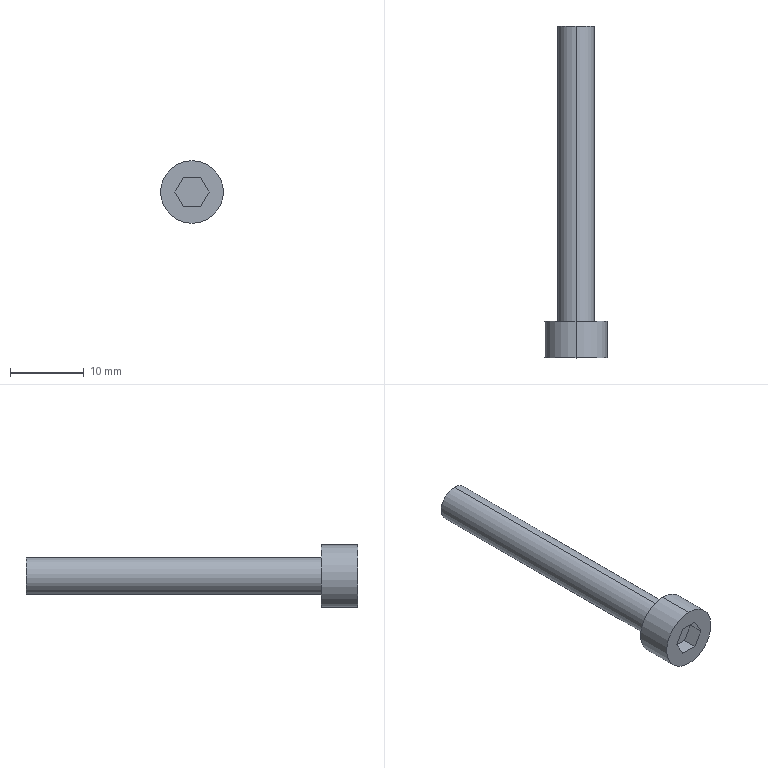Part | SolidWorks | features BaseBody 1 | 1 solid | 14 faces | box 8.5 x 45 x 8.5 mm | volume 1041 mm3 | plane 10 | cylinder 4 | commonest cylinder face diameters 5 x2 8.5 x2
STEP:
#1=CARTESIAN_POINT('',(0.,45.,-2.5));
#2=VERTEX_POINT('',#1);
#3=CARTESIAN_POINT('',(0.,45.,2.5));
#4=VERTEX_POINT('',#3);
#5=CARTESIAN_POINT('',(0.,45.,0.));
#6=DIRECTION('',(0.,-1.,0.));
#7=DIRECTION('',(0.,0.,-1.));
#8=AXIS2_PLACEMENT_3D('',#5,#6,#7);
#9=CIRCLE('',#8,2.5);
#10=EDGE_CURVE('',#2,#4,#9,.T.);
#11=ORIENTED_EDGE('',*,*,#10,.T.);
#12=CARTESIAN_POINT('',(0.,5.,2.5));
#13=VERTEX_POINT('',#12);
#14=CARTESIAN_POINT('',(0.,45.,2.5));
#15=DIRECTION('',(0.,-1.,0.));
#16=VECTOR('',#15,1000.);
#17=LINE('',#14,#16);
#18=EDGE_CURVE('',#4,#13,#17,.T.);
#19=ORIENTED_EDGE('',*,*,#18,.T.);
#20=CARTESIAN_POINT('',(0.,5.,-2.5));
#21=VERTEX_POINT('',#20);
#22=CARTESIAN_POINT('',(0.,5.,0.));
#23=DIRECTION('',(0.,1.,0.));
#24=DIRECTION('',(0.,0.,-1.));
#25=AXIS2_PLACEMENT_3D('',#22,#23,#24);
#26=CIRCLE('',#25,2.5);
#27=EDGE_CURVE('',#13,#21,#26,.T.);
#28=ORIENTED_EDGE('',*,*,#27,.T.);
#29=CARTESIAN_POINT('',(0.,45.,-2.5));
#30=DIRECTION('',(0.,-1.,0.));
#31=VECTOR('',#30,1000.);
#32=LINE('',#29,#31);
#33=EDGE_CURVE('',#2,#21,#32,.T.);
#34=ORIENTED_EDGE('',*,*,#33,.F.);
#35=EDGE_LOOP('',(#11,#19,#28,#34));
#36=FACE_OUTER_BOUND('',#35,.T.);
#37=CARTESIAN_POINT('',(0.,45.,0.));
#38=DIRECTION('',(0.,-1.,0.));
#39=DIRECTION('',(0.,0.,-1.));
#40=AXIS2_PLACEMENT_3D('',#37,#38,#39);
#41=CYLINDRICAL_SURFACE('',#40,2.5);
#42=ADVANCED_FACE('',(#36),#41,.T.);
#43=CARTESIAN_POINT('',(0.,5.,4.25));
#44=VERTEX_POINT('',#43);
#45=CARTESIAN_POINT('',(0.,5.,-4.25));
#46=VERTEX_POINT('',#45);
#47=CARTESIAN_POINT('',(0.,5.,0.));
#48=DIRECTION('',(0.,1.,0.));
#49=DIRECTION('',(0.,0.,-1.));
#50=AXIS2_PLACEMENT_3D('',#47,#48,#49);
#51=CIRCLE('',#50,4.25);
#52=EDGE_CURVE('',#44,#46,#51,.T.);
#53=ORIENTED_EDGE('',*,*,#52,.F.);
#54=CARTESIAN_POINT('',(0.,0.,4.25));
#55=VERTEX_POINT('',#54);
#56=CARTESIAN_POINT('',(0.,5.,4.25));
#57=DIRECTION('',(0.,-1.,0.));
#58=VECTOR('',#57,1000.);
#59=LINE('',#56,#58);
#60=EDGE_CURVE('',#44,#55,#59,.T.);
#61=ORIENTED_EDGE('',*,*,#60,.T.);
#62=CARTESIAN_POINT('',(0.,0.,-4.25));
#63=VERTEX_POINT('',#62);
#64=CARTESIAN_POINT('',(0.,0.,0.));
#65=DIRECTION('',(0.,1.,0.));
#66=DIRECTION('',(0.,0.,-1.));
#67=AXIS2_PLACEMENT_3D('',#64,#65,#66);
#68=CIRCLE('',#67,4.25);
#69=EDGE_CURVE('',#55,#63,#68,.T.);
#70=ORIENTED_EDGE('',*,*,#69,.T.);
#71=CARTESIAN_POINT('',(0.,5.,-4.25));
#72=DIRECTION('',(0.,-1.,0.));
#73=VECTOR('',#72,1000.);
#74=LINE('',#71,#73);
#75=EDGE_CURVE('',#46,#63,#74,.T.);
#76=ORIENTED_EDGE('',*,*,#75,.F.);
#77=EDGE_LOOP('',(#53,#61,#70,#76));
#78=FACE_OUTER_BOUND('',#77,.T.);
#79=CARTESIAN_POINT('',(0.,5.,0.));
#80=DIRECTION('',(0.,-1.,0.));
#81=DIRECTION('',(0.,0.,-1.));
#82=AXIS2_PLACEMENT_3D('',#79,#80,#81);
#83=CYLINDRICAL_SURFACE('',#82,4.25);
#84=ADVANCED_FACE('',(#78),#83,.T.);
#85=ORIENTED_EDGE('',*,*,#18,.F.);
#86=CARTESIAN_POINT('',(0.,45.,0.));
#87=DIRECTION('',(0.,-1.,0.));
#88=DIRECTION('',(0.,0.,-1.));
#89=AXIS2_PLACEMENT_3D('',#86,#87,#88);
#90=CIRCLE('',#89,2.5);
#91=EDGE_CURVE('',#4,#2,#90,.T.);
#92=ORIENTED_EDGE('',*,*,#91,.T.);
#93=ORIENTED_EDGE('',*,*,#33,.T.);
#94=CARTESIAN_POINT('',(0.,5.,0.));
#95=DIRECTION('',(0.,1.,0.));
#96=DIRECTION('',(0.,0.,-1.));
#97=AXIS2_PLACEMENT_3D('',#94,#95,#96);
#98=CIRCLE('',#97,2.5);
#99=EDGE_CURVE('',#21,#13,#98,.T.);
#100=ORIENTED_EDGE('',*,*,#99,.T.);
#101=EDGE_LOOP('',(#85,#92,#93,#100));
#102=FACE_OUTER_BOUND('',#101,.T.);
#103=CARTESIAN_POINT('',(0.,45.,0.));
#104=DIRECTION('',(0.,-1.,0.));
#105=DIRECTION('',(0.,0.,-1.));
#106=AXIS2_PLACEMENT_3D('',#103,#104,#105);
#107=CYLINDRICAL_SURFACE('',#106,2.5);
#108=ADVANCED_FACE('',(#102),#107,.T.);
#109=CARTESIAN_POINT('',(0.,5.,0.));
#110=DIRECTION('',(0.,1.,0.));
#111=DIRECTION('',(0.,0.,-1.));
#112=AXIS2_PLACEMENT_3D('',#109,#110,#111);
#113=CIRCLE('',#112,4.25);
#114=EDGE_CURVE('',#46,#44,#113,.T.);
#115=ORIENTED_EDGE('',*,*,#114,.T.);
#116=ORIENTED_EDGE('',*,*,#52,.T.);
#117=EDGE_LOOP('',(#115,#116));
#118=FACE_OUTER_BOUND('',#117,.T.);
#119=ORIENTED_EDGE('',*,*,#99,.F.);
#120=ORIENTED_EDGE('',*,*,#27,.F.);
#121=EDGE_LOOP('',(#119,#120));
#122=FACE_BOUND('',#121,.T.);
#123=CARTESIAN_POINT('',(0.,5.,0.));
#124=DIRECTION('',(0.,1.,0.));
#125=DIRECTION('',(0.,0.,1.));
#126=AXIS2_PLACEMENT_3D('',#123,#124,#125);
#127=PLANE('',#126);
#128=ADVANCED_FACE('',(#118,#122),#127,.T.);
#129=ORIENTED_EDGE('',*,*,#10,.F.);
#130=ORIENTED_EDGE('',*,*,#91,.F.);
#131=EDGE_LOOP('',(#129,#130));
#132=FACE_OUTER_BOUND('',#131,.T.);
#133=CARTESIAN_POINT('',(0.,45.,0.));
#134=DIRECTION('',(0.,1.,0.));
#135=DIRECTION('',(0.,0.,1.));
#136=AXIS2_PLACEMENT_3D('',#133,#134,#135);
#137=PLANE('',#136);
#138=ADVANCED_FACE('',(#132),#137,.T.);
#139=ORIENTED_EDGE('',*,*,#60,.F.);
#140=ORIENTED_EDGE('',*,*,#114,.F.);
#141=ORIENTED_EDGE('',*,*,#75,.T.);
#142=CARTESIAN_POINT('',(0.,0.,0.));
#143=DIRECTION('',(0.,1.,0.));
#144=DIRECTION('',(0.,0.,-1.));
#145=AXIS2_PLACEMENT_3D('',#142,#143,#144);
#146=CIRCLE('',#145,4.25);
#147=EDGE_CURVE('',#63,#55,#146,.T.);
#148=ORIENTED_EDGE('',*,*,#147,.T.);
#149=EDGE_LOOP('',(#139,#140,#141,#148));
#150=FACE_OUTER_BOUND('',#149,.T.);
#151=CARTESIAN_POINT('',(0.,5.,0.));
#152=DIRECTION('',(0.,-1.,0.));
#153=DIRECTION('',(0.,0.,-1.));
#154=AXIS2_PLACEMENT_3D('',#151,#152,#153);
#155=CYLINDRICAL_SURFACE('',#154,4.25);
#156=ADVANCED_FACE('',(#150),#155,.T.);
#157=ORIENTED_EDGE('',*,*,#147,.F.);
#158=ORIENTED_EDGE('',*,*,#69,.F.);
#159=EDGE_LOOP('',(#157,#158));
#160=FACE_OUTER_BOUND('',#159,.T.);
#161=CARTESIAN_POINT('',(1.155,0.,-2.));
#162=VERTEX_POINT('',#161);
#163=CARTESIAN_POINT('',(2.309,0.,0.));
#164=VERTEX_POINT('',#163);
#165=CARTESIAN_POINT('',(1.155,0.,-2.));
#166=DIRECTION('',(0.5,0.,0.866));
#167=VECTOR('',#166,1000.);
#168=LINE('',#165,#167);
#169=EDGE_CURVE('',#162,#164,#168,.T.);
#170=ORIENTED_EDGE('',*,*,#169,.F.);
#171=CARTESIAN_POINT('',(-1.155,0.,-2.));
#172=VERTEX_POINT('',#171);
#173=CARTESIAN_POINT('',(0.,0.,-2.));
#174=DIRECTION('',(1.,0.,0.));
#175=VECTOR('',#174,1000.);
#176=LINE('',#173,#175);
#177=EDGE_CURVE('',#172,#162,#176,.T.);
#178=ORIENTED_EDGE('',*,*,#177,.F.);
#179=CARTESIAN_POINT('',(-2.309,0.,0.));
#180=VERTEX_POINT('',#179);
#181=CARTESIAN_POINT('',(-2.309,0.,0.));
#182=DIRECTION('',(0.5,0.,-0.866));
#183=VECTOR('',#182,1000.);
#184=LINE('',#181,#183);
#185=EDGE_CURVE('',#180,#172,#184,.T.);
#186=ORIENTED_EDGE('',*,*,#185,.F.);
#187=CARTESIAN_POINT('',(-1.155,0.,2.));
#188=VERTEX_POINT('',#187);
#189=CARTESIAN_POINT('',(-1.155,0.,2.));
#190=DIRECTION('',(-0.5,0.,-0.866));
#191=VECTOR('',#190,1000.);
#192=LINE('',#189,#191);
#193=EDGE_CURVE('',#188,#180,#192,.T.);
#194=ORIENTED_EDGE('',*,*,#193,.F.);
#195=CARTESIAN_POINT('',(1.155,0.,2.));
#196=VERTEX_POINT('',#195);
#197=CARTESIAN_POINT('',(0.,0.,2.));
#198=DIRECTION('',(-1.,0.,0.));
#199=VECTOR('',#198,1000.);
#200=LINE('',#197,#199);
#201=EDGE_CURVE('',#196,#188,#200,.T.);
#202=ORIENTED_EDGE('',*,*,#201,.F.);
#203=CARTESIAN_POINT('',(2.309,0.,0.));
#204=DIRECTION('',(-0.5,0.,0.866));
#205=VECTOR('',#204,1000.);
#206=LINE('',#203,#205);
#207=EDGE_CURVE('',#164,#196,#206,.T.);
#208=ORIENTED_EDGE('',*,*,#207,.F.);
#209=EDGE_LOOP('',(#170,#178,#186,#194,#202,#208));
#210=FACE_BOUND('',#209,.T.);
#211=CARTESIAN_POINT('',(0.,0.,0.));
#212=DIRECTION('',(0.,1.,0.));
#213=DIRECTION('',(0.,0.,1.));
#214=AXIS2_PLACEMENT_3D('',#211,#212,#213);
#215=PLANE('',#214);
#216=ADVANCED_FACE('',(#160,#210),#215,.F.);
#217=CARTESIAN_POINT('',(1.155,2.,2.));
#218=VERTEX_POINT('',#217);
#219=CARTESIAN_POINT('',(1.155,2.,2.));
#220=DIRECTION('',(0.,-1.,0.));
#221=VECTOR('',#220,1000.);
#222=LINE('',#219,#221);
#223=EDGE_CURVE('',#218,#196,#222,.T.);
#224=ORIENTED_EDGE('',*,*,#223,.F.);
#225=CARTESIAN_POINT('',(2.309,2.,0.));
#226=VERTEX_POINT('',#225);
#227=CARTESIAN_POINT('',(2.309,2.,0.));
#228=DIRECTION('',(-0.5,0.,0.866));
#229=VECTOR('',#228,1000.);
#230=LINE('',#227,#229);
#231=EDGE_CURVE('',#226,#218,#230,.T.);
#232=ORIENTED_EDGE('',*,*,#231,.F.);
#233=CARTESIAN_POINT('',(2.309,2.,0.));
#234=DIRECTION('',(0.,1.,0.));
#235=VECTOR('',#234,1000.);
#236=LINE('',#233,#235);
#237=EDGE_CURVE('',#164,#226,#236,.T.);
#238=ORIENTED_EDGE('',*,*,#237,.F.);
#239=ORIENTED_EDGE('',*,*,#207,.T.);
#240=EDGE_LOOP('',(#224,#232,#238,#239));
#241=FACE_OUTER_BOUND('',#240,.T.);
#242=CARTESIAN_POINT('',(2.309,2.,0.));
#243=DIRECTION('',(0.866,0.,0.5));
#244=DIRECTION('',(0.5,0.,-0.866));
#245=AXIS2_PLACEMENT_3D('',#242,#243,#244);
#246=PLANE('',#245);
#247=ADVANCED_FACE('',(#241),#246,.F.);
#248=ORIENTED_EDGE('',*,*,#237,.T.);
#249=CARTESIAN_POINT('',(1.155,2.,-2.));
#250=VERTEX_POINT('',#249);
#251=CARTESIAN_POINT('',(1.155,2.,-2.));
#252=DIRECTION('',(0.5,0.,0.866));
#253=VECTOR('',#252,1000.);
#254=LINE('',#251,#253);
#255=EDGE_CURVE('',#250,#226,#254,.T.);
#256=ORIENTED_EDGE('',*,*,#255,.F.);
#257=CARTESIAN_POINT('',(1.155,2.,-2.));
#258=DIRECTION('',(0.,1.,0.));
#259=VECTOR('',#258,1000.);
#260=LINE('',#257,#259);
#261=EDGE_CURVE('',#162,#250,#260,.T.);
#262=ORIENTED_EDGE('',*,*,#261,.F.);
#263=ORIENTED_EDGE('',*,*,#169,.T.);
#264=EDGE_LOOP('',(#248,#256,#262,#263));
#265=FACE_OUTER_BOUND('',#264,.T.);
#266=CARTESIAN_POINT('',(1.155,2.,-2.));
#267=DIRECTION('',(0.866,0.,-0.5));
#268=DIRECTION('',(-0.5,0.,-0.866));
#269=AXIS2_PLACEMENT_3D('',#266,#267,#268);
#270=PLANE('',#269);
#271=ADVANCED_FACE('',(#265),#270,.F.);
#272=ORIENTED_EDGE('',*,*,#261,.T.);
#273=CARTESIAN_POINT('',(-1.155,2.,-2.));
#274=VERTEX_POINT('',#273);
#275=CARTESIAN_POINT('',(-1.155,2.,-2.));
#276=DIRECTION('',(1.,0.,0.));
#277=VECTOR('',#276,1000.);
#278=LINE('',#275,#277);
#279=EDGE_CURVE('',#274,#250,#278,.T.);
#280=ORIENTED_EDGE('',*,*,#279,.F.);
#281=CARTESIAN_POINT('',(-1.155,2.,-2.));
#282=DIRECTION('',(0.,1.,0.));
#283=VECTOR('',#282,1000.);
#284=LINE('',#281,#283);
#285=EDGE_CURVE('',#172,#274,#284,.T.);
#286=ORIENTED_EDGE('',*,*,#285,.F.);
#287=ORIENTED_EDGE('',*,*,#177,.T.);
#288=EDGE_LOOP('',(#272,#280,#286,#287));
#289=FACE_OUTER_BOUND('',#288,.T.);
#290=CARTESIAN_POINT('',(-1.155,2.,-2.));
#291=DIRECTION('',(0.,0.,-1.));
#292=DIRECTION('',(-1.,0.,0.));
#293=AXIS2_PLACEMENT_3D('',#290,#291,#292);
#294=PLANE('',#293);
#295=ADVANCED_FACE('',(#289),#294,.F.);
#296=ORIENTED_EDGE('',*,*,#285,.T.);
#297=CARTESIAN_POINT('',(-2.309,2.,0.));
#298=VERTEX_POINT('',#297);
#299=CARTESIAN_POINT('',(-2.309,2.,0.));
#300=DIRECTION('',(0.5,0.,-0.866));
#301=VECTOR('',#300,1000.);
#302=LINE('',#299,#301);
#303=EDGE_CURVE('',#298,#274,#302,.T.);
#304=ORIENTED_EDGE('',*,*,#303,.F.);
#305=CARTESIAN_POINT('',(-2.309,2.,0.));
#306=DIRECTION('',(0.,1.,0.));
#307=VECTOR('',#306,1000.);
#308=LINE('',#305,#307);
#309=EDGE_CURVE('',#180,#298,#308,.T.);
#310=ORIENTED_EDGE('',*,*,#309,.F.);
#311=ORIENTED_EDGE('',*,*,#185,.T.);
#312=EDGE_LOOP('',(#296,#304,#310,#311));
#313=FACE_OUTER_BOUND('',#312,.T.);
#314=CARTESIAN_POINT('',(-2.309,2.,0.));
#315=DIRECTION('',(-0.866,0.,-0.5));
#316=DIRECTION('',(-0.5,0.,0.866));
#317=AXIS2_PLACEMENT_3D('',#314,#315,#316);
#318=PLANE('',#317);
#319=ADVANCED_FACE('',(#313),#318,.F.);
#320=ORIENTED_EDGE('',*,*,#309,.T.);
#321=CARTESIAN_POINT('',(-1.155,2.,2.));
#322=VERTEX_POINT('',#321);
#323=CARTESIAN_POINT('',(-1.155,2.,2.));
#324=DIRECTION('',(-0.5,0.,-0.866));
#325=VECTOR('',#324,1000.);
#326=LINE('',#323,#325);
#327=EDGE_CURVE('',#322,#298,#326,.T.);
#328=ORIENTED_EDGE('',*,*,#327,.F.);
#329=CARTESIAN_POINT('',(-1.155,2.,2.));
#330=DIRECTION('',(0.,1.,0.));
#331=VECTOR('',#330,1000.);
#332=LINE('',#329,#331);
#333=EDGE_CURVE('',#188,#322,#332,.T.);
#334=ORIENTED_EDGE('',*,*,#333,.F.);
#335=ORIENTED_EDGE('',*,*,#193,.T.);
#336=EDGE_LOOP('',(#320,#328,#334,#335));
#337=FACE_OUTER_BOUND('',#336,.T.);
#338=CARTESIAN_POINT('',(-1.155,2.,2.));
#339=DIRECTION('',(-0.866,0.,0.5));
#340=DIRECTION('',(0.5,0.,0.866));
#341=AXIS2_PLACEMENT_3D('',#338,#339,#340);
#342=PLANE('',#341);
#343=ADVANCED_FACE('',(#337),#342,.F.);
#344=ORIENTED_EDGE('',*,*,#333,.T.);
#345=CARTESIAN_POINT('',(1.155,2.,2.));
#346=DIRECTION('',(-1.,0.,0.));
#347=VECTOR('',#346,1000.);
#348=LINE('',#345,#347);
#349=EDGE_CURVE('',#218,#322,#348,.T.);
#350=ORIENTED_EDGE('',*,*,#349,.F.);
#351=ORIENTED_EDGE('',*,*,#223,.T.);
#352=ORIENTED_EDGE('',*,*,#201,.T.);
#353=EDGE_LOOP('',(#344,#350,#351,#352));
#354=FACE_OUTER_BOUND('',#353,.T.);
#355=CARTESIAN_POINT('',(1.155,2.,2.));
#356=DIRECTION('',(0.,0.,1.));
#357=DIRECTION('',(1.,0.,0.));
#358=AXIS2_PLACEMENT_3D('',#355,#356,#357);
#359=PLANE('',#358);
#360=ADVANCED_FACE('',(#354),#359,.F.);
#361=ORIENTED_EDGE('',*,*,#303,.T.);
#362=ORIENTED_EDGE('',*,*,#279,.T.);
#363=ORIENTED_EDGE('',*,*,#255,.T.);
#364=ORIENTED_EDGE('',*,*,#231,.T.);
#365=ORIENTED_EDGE('',*,*,#349,.T.);
#366=ORIENTED_EDGE('',*,*,#327,.T.);
#367=EDGE_LOOP('',(#361,#362,#363,#364,#365,#366));
#368=FACE_OUTER_BOUND('',#367,.T.);
#369=CARTESIAN_POINT('',(0.,2.,0.));
#370=DIRECTION('',(0.,-1.,0.));
#371=DIRECTION('',(0.,0.,-1.));
#372=AXIS2_PLACEMENT_3D('',#369,#370,#371);
#373=PLANE('',#372);
#374=ADVANCED_FACE('',(#368),#373,.T.);
#375=CLOSED_SHELL('',(#42,#84,#108,#128,#138,#156,#216,#247,#271,#295,#319,#343,#360,#374));
#376=MANIFOLD_SOLID_BREP('',#375);
#377=CARTESIAN_POINT('',(0.,0.,0.));
#378=DIRECTION('',(0.,0.,1.));
#379=DIRECTION('',(1.,0.,0.));
#380=AXIS2_PLACEMENT_3D('',#377,#378,#379);
#381=(LENGTH_UNIT()NAMED_UNIT(*)SI_UNIT(.MILLI.,.METRE.));
#382=UNCERTAINTY_MEASURE_WITH_UNIT(LENGTH_MEASURE(0.00001),#381,'','');
#383=(NAMED_UNIT(*)PLANE_ANGLE_UNIT()SI_UNIT($,.RADIAN.));
#384=(NAMED_UNIT(*)SI_UNIT($,.STERADIAN.)SOLID_ANGLE_UNIT());
#385=(GEOMETRIC_REPRESENTATION_CONTEXT(3)GLOBAL_UNCERTAINTY_ASSIGNED_CONTEXT((#382))GLOBAL_UNIT_ASSIGNED_CONTEXT((#381,#383,#384))REPRESENTATION_CONTEXT('',''));
#386=ADVANCED_BREP_SHAPE_REPRESENTATION('',(#376,#380),#385);